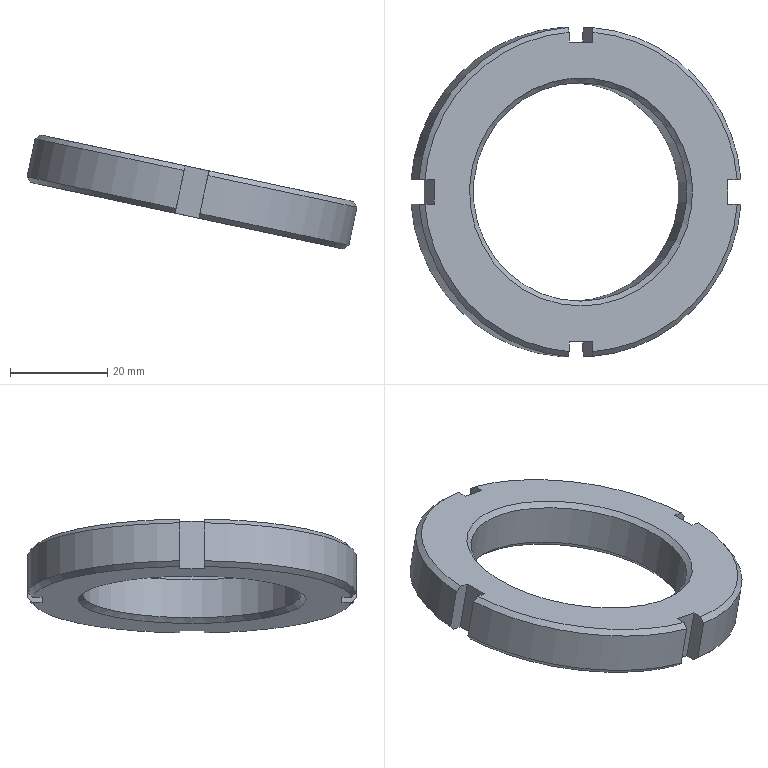Part | STEP file | HL4GZ-1.862.557 (lock nut) | 1 solid | 29 faces | box 67.997 x 67.816 x 23.464 mm | volume 19464 mm3 | plane 14 | cone 10 | cylinder 5 | commonest cylinder face diameters 68 x4 45 x1